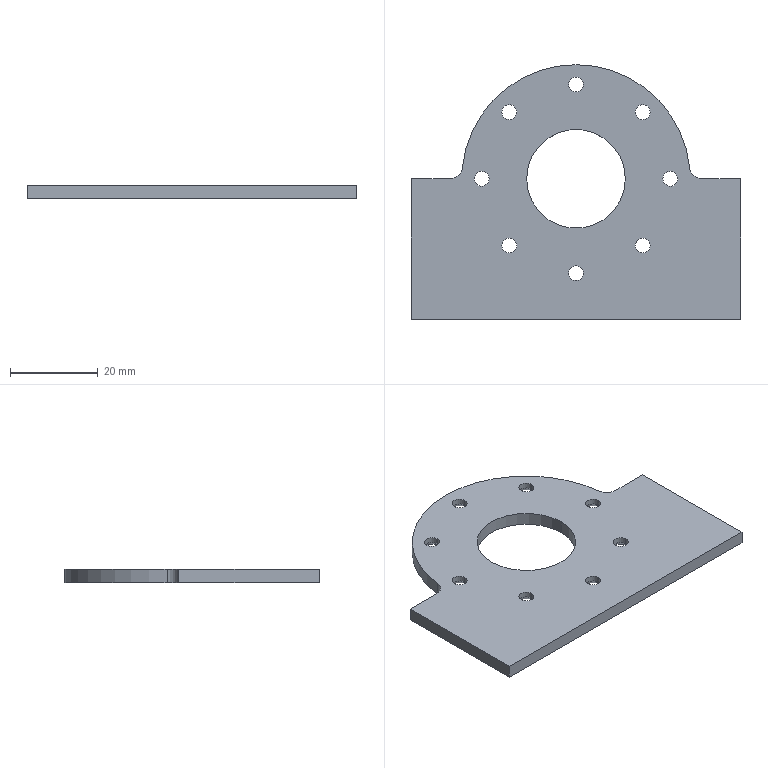Part | SolidWorks | features ICE 2, Extrusion 1, Fillet 1, HoleWzd 1 | 1 solid | 44 faces | box 75 x 58 x 3 mm | volume 8829 mm3 | cylinder 21 | cone 16 | plane 7 | commonest cylinder face diameters 3.4 x16 6 x2 22.5 x2 52 x1
STEP:
#1=CARTESIAN_POINT('',(1.7,37.5,1.66));
#2=VERTEX_POINT('',#1);
#3=CARTESIAN_POINT('',(-1.7,37.5,1.66));
#4=VERTEX_POINT('',#3);
#5=CARTESIAN_POINT('',(0.,37.5,1.66));
#6=DIRECTION('',(0.,0.,-1.));
#7=DIRECTION('',(-1.,0.,0.));
#8=AXIS2_PLACEMENT_3D('',#5,#6,#7);
#9=CIRCLE('',#8,1.7);
#10=EDGE_CURVE('',#2,#4,#9,.T.);
#11=ORIENTED_EDGE('',*,*,#10,.F.);
#12=CARTESIAN_POINT('',(3.36,37.5,0.));
#13=VERTEX_POINT('',#12);
#14=CARTESIAN_POINT('',(3.36,37.5,0.));
#15=DIRECTION('',(0.7071,0.,-0.7071));
#16=VECTOR('',#15,1000.);
#17=LINE('',#14,#16);
#18=EDGE_CURVE('',#2,#13,#17,.T.);
#19=ORIENTED_EDGE('',*,*,#18,.T.);
#20=CARTESIAN_POINT('',(-3.36,37.5,0.));
#21=VERTEX_POINT('',#20);
#22=CARTESIAN_POINT('',(0.,37.5,0.));
#23=DIRECTION('',(0.,0.,-1.));
#24=DIRECTION('',(-1.,0.,0.));
#25=AXIS2_PLACEMENT_3D('',#22,#23,#24);
#26=CIRCLE('',#25,3.36);
#27=EDGE_CURVE('',#13,#21,#26,.T.);
#28=ORIENTED_EDGE('',*,*,#27,.T.);
#29=CARTESIAN_POINT('',(-3.36,37.5,0.));
#30=DIRECTION('',(-0.7071,0.,-0.7071));
#31=VECTOR('',#30,1000.);
#32=LINE('',#29,#31);
#33=EDGE_CURVE('',#4,#21,#32,.T.);
#34=ORIENTED_EDGE('',*,*,#33,.F.);
#35=EDGE_LOOP('',(#11,#19,#28,#34));
#36=FACE_OUTER_BOUND('',#35,.T.);
#37=CARTESIAN_POINT('',(0.,37.5,0.));
#38=DIRECTION('',(0.,0.,-1.));
#39=DIRECTION('',(-1.,0.,0.));
#40=AXIS2_PLACEMENT_3D('',#37,#38,#39);
#41=CONICAL_SURFACE('',#40,3.36,0.7854);
#42=ADVANCED_FACE('',(#36),#41,.F.);
#43=CARTESIAN_POINT('',(1.7,37.5,3.));
#44=VERTEX_POINT('',#43);
#45=CARTESIAN_POINT('',(-1.7,37.5,3.));
#46=VERTEX_POINT('',#45);
#47=CARTESIAN_POINT('',(0.,37.5,3.));
#48=DIRECTION('',(0.,0.,-1.));
#49=DIRECTION('',(-1.,0.,0.));
#50=AXIS2_PLACEMENT_3D('',#47,#48,#49);
#51=CIRCLE('',#50,1.7);
#52=EDGE_CURVE('',#44,#46,#51,.T.);
#53=ORIENTED_EDGE('',*,*,#52,.F.);
#54=CARTESIAN_POINT('',(1.7,37.5,0.));
#55=DIRECTION('',(0.,0.,-1.));
#56=VECTOR('',#55,1000.);
#57=LINE('',#54,#56);
#58=EDGE_CURVE('',#44,#2,#57,.T.);
#59=ORIENTED_EDGE('',*,*,#58,.T.);
#60=ORIENTED_EDGE('',*,*,#10,.T.);
#61=CARTESIAN_POINT('',(-1.7,37.5,0.));
#62=DIRECTION('',(0.,0.,-1.));
#63=VECTOR('',#62,1000.);
#64=LINE('',#61,#63);
#65=EDGE_CURVE('',#46,#4,#64,.T.);
#66=ORIENTED_EDGE('',*,*,#65,.F.);
#67=EDGE_LOOP('',(#53,#59,#60,#66));
#68=FACE_OUTER_BOUND('',#67,.T.);
#69=CARTESIAN_POINT('',(0.,37.5,0.));
#70=DIRECTION('',(0.,0.,-1.));
#71=DIRECTION('',(-1.,0.,0.));
#72=AXIS2_PLACEMENT_3D('',#69,#70,#71);
#73=CYLINDRICAL_SURFACE('',#72,1.7);
#74=ADVANCED_FACE('',(#68),#73,.F.);
#75=CARTESIAN_POINT('',(-13.503,31.203,1.66));
#76=VERTEX_POINT('',#75);
#77=CARTESIAN_POINT('',(-16.903,31.203,1.66));
#78=VERTEX_POINT('',#77);
#79=CARTESIAN_POINT('',(-15.203,31.203,1.66));
#80=DIRECTION('',(0.,0.,-1.));
#81=DIRECTION('',(-1.,0.,0.));
#82=AXIS2_PLACEMENT_3D('',#79,#80,#81);
#83=CIRCLE('',#82,1.7);
#84=EDGE_CURVE('',#76,#78,#83,.T.);
#85=ORIENTED_EDGE('',*,*,#84,.F.);
#86=CARTESIAN_POINT('',(-11.843,31.203,0.));
#87=VERTEX_POINT('',#86);
#88=CARTESIAN_POINT('',(-11.843,31.203,0.));
#89=DIRECTION('',(0.7071,0.,-0.7071));
#90=VECTOR('',#89,1000.);
#91=LINE('',#88,#90);
#92=EDGE_CURVE('',#76,#87,#91,.T.);
#93=ORIENTED_EDGE('',*,*,#92,.T.);
#94=CARTESIAN_POINT('',(-18.563,31.203,0.));
#95=VERTEX_POINT('',#94);
#96=CARTESIAN_POINT('',(-15.203,31.203,0.));
#97=DIRECTION('',(0.,0.,-1.));
#98=DIRECTION('',(-1.,0.,0.));
#99=AXIS2_PLACEMENT_3D('',#96,#97,#98);
#100=CIRCLE('',#99,3.36);
#101=EDGE_CURVE('',#87,#95,#100,.T.);
#102=ORIENTED_EDGE('',*,*,#101,.T.);
#103=CARTESIAN_POINT('',(-18.563,31.203,0.));
#104=DIRECTION('',(-0.7071,0.,-0.7071));
#105=VECTOR('',#104,1000.);
#106=LINE('',#103,#105);
#107=EDGE_CURVE('',#78,#95,#106,.T.);
#108=ORIENTED_EDGE('',*,*,#107,.F.);
#109=EDGE_LOOP('',(#85,#93,#102,#108));
#110=FACE_OUTER_BOUND('',#109,.T.);
#111=CARTESIAN_POINT('',(-15.203,31.203,0.));
#112=DIRECTION('',(0.,0.,-1.));
#113=DIRECTION('',(-1.,0.,0.));
#114=AXIS2_PLACEMENT_3D('',#111,#112,#113);
#115=CONICAL_SURFACE('',#114,3.36,0.7854);
#116=ADVANCED_FACE('',(#110),#115,.F.);
#117=CARTESIAN_POINT('',(-13.503,31.203,3.));
#118=VERTEX_POINT('',#117);
#119=CARTESIAN_POINT('',(-16.903,31.203,3.));
#120=VERTEX_POINT('',#119);
#121=CARTESIAN_POINT('',(-15.203,31.203,3.));
#122=DIRECTION('',(0.,0.,-1.));
#123=DIRECTION('',(-1.,0.,0.));
#124=AXIS2_PLACEMENT_3D('',#121,#122,#123);
#125=CIRCLE('',#124,1.7);
#126=EDGE_CURVE('',#118,#120,#125,.T.);
#127=ORIENTED_EDGE('',*,*,#126,.F.);
#128=CARTESIAN_POINT('',(-13.503,31.203,0.));
#129=DIRECTION('',(0.,0.,-1.));
#130=VECTOR('',#129,1000.);
#131=LINE('',#128,#130);
#132=EDGE_CURVE('',#118,#76,#131,.T.);
#133=ORIENTED_EDGE('',*,*,#132,.T.);
#134=ORIENTED_EDGE('',*,*,#84,.T.);
#135=CARTESIAN_POINT('',(-16.903,31.203,0.));
#136=DIRECTION('',(0.,0.,-1.));
#137=VECTOR('',#136,1000.);
#138=LINE('',#135,#137);
#139=EDGE_CURVE('',#120,#78,#138,.T.);
#140=ORIENTED_EDGE('',*,*,#139,.F.);
#141=EDGE_LOOP('',(#127,#133,#134,#140));
#142=FACE_OUTER_BOUND('',#141,.T.);
#143=CARTESIAN_POINT('',(-15.203,31.203,0.));
#144=DIRECTION('',(0.,0.,-1.));
#145=DIRECTION('',(-1.,0.,0.));
#146=AXIS2_PLACEMENT_3D('',#143,#144,#145);
#147=CYLINDRICAL_SURFACE('',#146,1.7);
#148=ADVANCED_FACE('',(#142),#147,.F.);
#149=CARTESIAN_POINT('',(-19.8,16.,1.66));
#150=VERTEX_POINT('',#149);
#151=CARTESIAN_POINT('',(-23.2,16.,1.66));
#152=VERTEX_POINT('',#151);
#153=CARTESIAN_POINT('',(-21.5,16.,1.66));
#154=DIRECTION('',(0.,0.,-1.));
#155=DIRECTION('',(-1.,0.,0.));
#156=AXIS2_PLACEMENT_3D('',#153,#154,#155);
#157=CIRCLE('',#156,1.7);
#158=EDGE_CURVE('',#150,#152,#157,.T.);
#159=ORIENTED_EDGE('',*,*,#158,.F.);
#160=CARTESIAN_POINT('',(-18.14,16.,0.));
#161=VERTEX_POINT('',#160);
#162=CARTESIAN_POINT('',(-18.14,16.,0.));
#163=DIRECTION('',(0.7071,0.,-0.7071));
#164=VECTOR('',#163,1000.);
#165=LINE('',#162,#164);
#166=EDGE_CURVE('',#150,#161,#165,.T.);
#167=ORIENTED_EDGE('',*,*,#166,.T.);
#168=CARTESIAN_POINT('',(-24.86,16.,0.));
#169=VERTEX_POINT('',#168);
#170=CARTESIAN_POINT('',(-21.5,16.,0.));
#171=DIRECTION('',(0.,0.,-1.));
#172=DIRECTION('',(-1.,0.,0.));
#173=AXIS2_PLACEMENT_3D('',#170,#171,#172);
#174=CIRCLE('',#173,3.36);
#175=EDGE_CURVE('',#161,#169,#174,.T.);
#176=ORIENTED_EDGE('',*,*,#175,.T.);
#177=CARTESIAN_POINT('',(-24.86,16.,0.));
#178=DIRECTION('',(-0.7071,0.,-0.7071));
#179=VECTOR('',#178,1000.);
#180=LINE('',#177,#179);
#181=EDGE_CURVE('',#152,#169,#180,.T.);
#182=ORIENTED_EDGE('',*,*,#181,.F.);
#183=EDGE_LOOP('',(#159,#167,#176,#182));
#184=FACE_OUTER_BOUND('',#183,.T.);
#185=CARTESIAN_POINT('',(-21.5,16.,0.));
#186=DIRECTION('',(0.,0.,-1.));
#187=DIRECTION('',(-1.,0.,0.));
#188=AXIS2_PLACEMENT_3D('',#185,#186,#187);
#189=CONICAL_SURFACE('',#188,3.36,0.7854);
#190=ADVANCED_FACE('',(#184),#189,.F.);
#191=CARTESIAN_POINT('',(-19.8,16.,3.));
#192=VERTEX_POINT('',#191);
#193=CARTESIAN_POINT('',(-23.2,16.,3.));
#194=VERTEX_POINT('',#193);
#195=CARTESIAN_POINT('',(-21.5,16.,3.));
#196=DIRECTION('',(0.,0.,-1.));
#197=DIRECTION('',(-1.,0.,0.));
#198=AXIS2_PLACEMENT_3D('',#195,#196,#197);
#199=CIRCLE('',#198,1.7);
#200=EDGE_CURVE('',#192,#194,#199,.T.);
#201=ORIENTED_EDGE('',*,*,#200,.F.);
#202=CARTESIAN_POINT('',(-19.8,16.,0.));
#203=DIRECTION('',(0.,0.,-1.));
#204=VECTOR('',#203,1000.);
#205=LINE('',#202,#204);
#206=EDGE_CURVE('',#192,#150,#205,.T.);
#207=ORIENTED_EDGE('',*,*,#206,.T.);
#208=ORIENTED_EDGE('',*,*,#158,.T.);
#209=CARTESIAN_POINT('',(-23.2,16.,0.));
#210=DIRECTION('',(0.,0.,-1.));
#211=VECTOR('',#210,1000.);
#212=LINE('',#209,#211);
#213=EDGE_CURVE('',#194,#152,#212,.T.);
#214=ORIENTED_EDGE('',*,*,#213,.F.);
#215=EDGE_LOOP('',(#201,#207,#208,#214));
#216=FACE_OUTER_BOUND('',#215,.T.);
#217=CARTESIAN_POINT('',(-21.5,16.,0.));
#218=DIRECTION('',(0.,0.,-1.));
#219=DIRECTION('',(-1.,0.,0.));
#220=AXIS2_PLACEMENT_3D('',#217,#218,#219);
#221=CYLINDRICAL_SURFACE('',#220,1.7);
#222=ADVANCED_FACE('',(#216),#221,.F.);
#223=CARTESIAN_POINT('',(-13.503,0.7972,1.66));
#224=VERTEX_POINT('',#223);
#225=CARTESIAN_POINT('',(-16.903,0.7972,1.66));
#226=VERTEX_POINT('',#225);
#227=CARTESIAN_POINT('',(-15.203,0.7972,1.66));
#228=DIRECTION('',(0.,0.,-1.));
#229=DIRECTION('',(-1.,0.,0.));
#230=AXIS2_PLACEMENT_3D('',#227,#228,#229);
#231=CIRCLE('',#230,1.7);
#232=EDGE_CURVE('',#224,#226,#231,.T.);
#233=ORIENTED_EDGE('',*,*,#232,.F.);
#234=CARTESIAN_POINT('',(-11.843,0.7972,0.));
#235=VERTEX_POINT('',#234);
#236=CARTESIAN_POINT('',(-11.843,0.7972,0.));
#237=DIRECTION('',(0.7071,0.,-0.7071));
#238=VECTOR('',#237,1000.);
#239=LINE('',#236,#238);
#240=EDGE_CURVE('',#224,#235,#239,.T.);
#241=ORIENTED_EDGE('',*,*,#240,.T.);
#242=CARTESIAN_POINT('',(-18.563,0.7972,0.));
#243=VERTEX_POINT('',#242);
#244=CARTESIAN_POINT('',(-15.203,0.7972,0.));
#245=DIRECTION('',(0.,0.,-1.));
#246=DIRECTION('',(-1.,0.,0.));
#247=AXIS2_PLACEMENT_3D('',#244,#245,#246);
#248=CIRCLE('',#247,3.36);
#249=EDGE_CURVE('',#235,#243,#248,.T.);
#250=ORIENTED_EDGE('',*,*,#249,.T.);
#251=CARTESIAN_POINT('',(-18.563,0.7972,0.));
#252=DIRECTION('',(-0.7071,0.,-0.7071));
#253=VECTOR('',#252,1000.);
#254=LINE('',#251,#253);
#255=EDGE_CURVE('',#226,#243,#254,.T.);
#256=ORIENTED_EDGE('',*,*,#255,.F.);
#257=EDGE_LOOP('',(#233,#241,#250,#256));
#258=FACE_OUTER_BOUND('',#257,.T.);
#259=CARTESIAN_POINT('',(-15.203,0.7972,0.));
#260=DIRECTION('',(0.,0.,-1.));
#261=DIRECTION('',(-1.,0.,0.));
#262=AXIS2_PLACEMENT_3D('',#259,#260,#261);
#263=CONICAL_SURFACE('',#262,3.36,0.7854);
#264=ADVANCED_FACE('',(#258),#263,.F.);
#265=CARTESIAN_POINT('',(-13.503,0.7972,3.));
#266=VERTEX_POINT('',#265);
#267=CARTESIAN_POINT('',(-16.903,0.7972,3.));
#268=VERTEX_POINT('',#267);
#269=CARTESIAN_POINT('',(-15.203,0.7972,3.));
#270=DIRECTION('',(0.,0.,-1.));
#271=DIRECTION('',(-1.,0.,0.));
#272=AXIS2_PLACEMENT_3D('',#269,#270,#271);
#273=CIRCLE('',#272,1.7);
#274=EDGE_CURVE('',#266,#268,#273,.T.);
#275=ORIENTED_EDGE('',*,*,#274,.F.);
#276=CARTESIAN_POINT('',(-13.503,0.7972,0.));
#277=DIRECTION('',(0.,0.,-1.));
#278=VECTOR('',#277,1000.);
#279=LINE('',#276,#278);
#280=EDGE_CURVE('',#266,#224,#279,.T.);
#281=ORIENTED_EDGE('',*,*,#280,.T.);
#282=ORIENTED_EDGE('',*,*,#232,.T.);
#283=CARTESIAN_POINT('',(-16.903,0.7972,0.));
#284=DIRECTION('',(0.,0.,-1.));
#285=VECTOR('',#284,1000.);
#286=LINE('',#283,#285);
#287=EDGE_CURVE('',#268,#226,#286,.T.);
#288=ORIENTED_EDGE('',*,*,#287,.F.);
#289=EDGE_LOOP('',(#275,#281,#282,#288));
#290=FACE_OUTER_BOUND('',#289,.T.);
#291=CARTESIAN_POINT('',(-15.203,0.7972,0.));
#292=DIRECTION('',(0.,0.,-1.));
#293=DIRECTION('',(-1.,0.,0.));
#294=AXIS2_PLACEMENT_3D('',#291,#292,#293);
#295=CYLINDRICAL_SURFACE('',#294,1.7);
#296=ADVANCED_FACE('',(#290),#295,.F.);
#297=CARTESIAN_POINT('',(1.7,-5.5,1.66));
#298=VERTEX_POINT('',#297);
#299=CARTESIAN_POINT('',(-1.7,-5.5,1.66));
#300=VERTEX_POINT('',#299);
#301=CARTESIAN_POINT('',(0.,-5.5,1.66));
#302=DIRECTION('',(0.,0.,-1.));
#303=DIRECTION('',(-1.,0.,0.));
#304=AXIS2_PLACEMENT_3D('',#301,#302,#303);
#305=CIRCLE('',#304,1.7);
#306=EDGE_CURVE('',#298,#300,#305,.T.);
#307=ORIENTED_EDGE('',*,*,#306,.F.);
#308=CARTESIAN_POINT('',(3.36,-5.5,0.));
#309=VERTEX_POINT('',#308);
#310=CARTESIAN_POINT('',(3.36,-5.5,0.));
#311=DIRECTION('',(0.7071,0.,-0.7071));
#312=VECTOR('',#311,1000.);
#313=LINE('',#310,#312);
#314=EDGE_CURVE('',#298,#309,#313,.T.);
#315=ORIENTED_EDGE('',*,*,#314,.T.);
#316=CARTESIAN_POINT('',(-3.36,-5.5,0.));
#317=VERTEX_POINT('',#316);
#318=CARTESIAN_POINT('',(0.,-5.5,0.));
#319=DIRECTION('',(0.,0.,-1.));
#320=DIRECTION('',(-1.,0.,0.));
#321=AXIS2_PLACEMENT_3D('',#318,#319,#320);
#322=CIRCLE('',#321,3.36);
#323=EDGE_CURVE('',#309,#317,#322,.T.);
#324=ORIENTED_EDGE('',*,*,#323,.T.);
#325=CARTESIAN_POINT('',(-3.36,-5.5,0.));
#326=DIRECTION('',(-0.7071,0.,-0.7071));
#327=VECTOR('',#326,1000.);
#328=LINE('',#325,#327);
#329=EDGE_CURVE('',#300,#317,#328,.T.);
#330=ORIENTED_EDGE('',*,*,#329,.F.);
#331=EDGE_LOOP('',(#307,#315,#324,#330));
#332=FACE_OUTER_BOUND('',#331,.T.);
#333=CARTESIAN_POINT('',(0.,-5.5,0.));
#334=DIRECTION('',(0.,0.,-1.));
#335=DIRECTION('',(-1.,0.,0.));
#336=AXIS2_PLACEMENT_3D('',#333,#334,#335);
#337=CONICAL_SURFACE('',#336,3.36,0.7854);
#338=ADVANCED_FACE('',(#332),#337,.F.);
#339=CARTESIAN_POINT('',(1.7,-5.5,3.));
#340=VERTEX_POINT('',#339);
#341=CARTESIAN_POINT('',(-1.7,-5.5,3.));
#342=VERTEX_POINT('',#341);
#343=CARTESIAN_POINT('',(0.,-5.5,3.));
#344=DIRECTION('',(0.,0.,-1.));
#345=DIRECTION('',(-1.,0.,0.));
#346=AXIS2_PLACEMENT_3D('',#343,#344,#345);
#347=CIRCLE('',#346,1.7);
#348=EDGE_CURVE('',#340,#342,#347,.T.);
#349=ORIENTED_EDGE('',*,*,#348,.F.);
#350=CARTESIAN_POINT('',(1.7,-5.5,0.));
#351=DIRECTION('',(0.,0.,-1.));
#352=VECTOR('',#351,1000.);
#353=LINE('',#350,#352);
#354=EDGE_CURVE('',#340,#298,#353,.T.);
#355=ORIENTED_EDGE('',*,*,#354,.T.);
#356=ORIENTED_EDGE('',*,*,#306,.T.);
#357=CARTESIAN_POINT('',(-1.7,-5.5,0.));
#358=DIRECTION('',(0.,0.,-1.));
#359=VECTOR('',#358,1000.);
#360=LINE('',#357,#359);
#361=EDGE_CURVE('',#342,#300,#360,.T.);
#362=ORIENTED_EDGE('',*,*,#361,.F.);
#363=EDGE_LOOP('',(#349,#355,#356,#362));
#364=FACE_OUTER_BOUND('',#363,.T.);
#365=CARTESIAN_POINT('',(0.,-5.5,0.));
#366=DIRECTION('',(0.,0.,-1.));
#367=DIRECTION('',(-1.,0.,0.));
#368=AXIS2_PLACEMENT_3D('',#365,#366,#367);
#369=CYLINDRICAL_SURFACE('',#368,1.7);
#370=ADVANCED_FACE('',(#364),#369,.F.);
#371=CARTESIAN_POINT('',(16.903,0.7972,1.66));
#372=VERTEX_POINT('',#371);
#373=CARTESIAN_POINT('',(13.503,0.7972,1.66));
#374=VERTEX_POINT('',#373);
#375=CARTESIAN_POINT('',(15.203,0.7972,1.66));
#376=DIRECTION('',(0.,0.,-1.));
#377=DIRECTION('',(-1.,0.,0.));
#378=AXIS2_PLACEMENT_3D('',#375,#376,#377);
#379=CIRCLE('',#378,1.7);
#380=EDGE_CURVE('',#372,#374,#379,.T.);
#381=ORIENTED_EDGE('',*,*,#380,.F.);
#382=CARTESIAN_POINT('',(18.563,0.7972,0.));
#383=VERTEX_POINT('',#382);
#384=CARTESIAN_POINT('',(18.563,0.7972,0.));
#385=DIRECTION('',(0.7071,0.,-0.7071));
#386=VECTOR('',#385,1000.);
#387=LINE('',#384,#386);
#388=EDGE_CURVE('',#372,#383,#387,.T.);
#389=ORIENTED_EDGE('',*,*,#388,.T.);
#390=CARTESIAN_POINT('',(11.843,0.7972,0.));
#391=VERTEX_POINT('',#390);
#392=CARTESIAN_POINT('',(15.203,0.7972,0.));
#393=DIRECTION('',(0.,0.,-1.));
#394=DIRECTION('',(-1.,0.,0.));
#395=AXIS2_PLACEMENT_3D('',#392,#393,#394);
#396=CIRCLE('',#395,3.36);
#397=EDGE_CURVE('',#383,#391,#396,.T.);
#398=ORIENTED_EDGE('',*,*,#397,.T.);
#399=CARTESIAN_POINT('',(11.843,0.7972,0.));
#400=DIRECTION('',(-0.7071,0.,-0.7071));
#401=VECTOR('',#400,1000.);
#402=LINE('',#399,#401);
#403=EDGE_CURVE('',#374,#391,#402,.T.);
#404=ORIENTED_EDGE('',*,*,#403,.F.);
#405=EDGE_LOOP('',(#381,#389,#398,#404));
#406=FACE_OUTER_BOUND('',#405,.T.);
#407=CARTESIAN_POINT('',(15.203,0.7972,0.));
#408=DIRECTION('',(0.,0.,-1.));
#409=DIRECTION('',(-1.,0.,0.));
#410=AXIS2_PLACEMENT_3D('',#407,#408,#409);
#411=CONICAL_SURFACE('',#410,3.36,0.7854);
#412=ADVANCED_FACE('',(#406),#411,.F.);
#413=CARTESIAN_POINT('',(16.903,0.7972,3.));
#414=VERTEX_POINT('',#413);
#415=CARTESIAN_POINT('',(13.503,0.7972,3.));
#416=VERTEX_POINT('',#415);
#417=CARTESIAN_POINT('',(15.203,0.7972,3.));
#418=DIRECTION('',(0.,0.,-1.));
#419=DIRECTION('',(-1.,0.,0.));
#420=AXIS2_PLACEMENT_3D('',#417,#418,#419);
#421=CIRCLE('',#420,1.7);
#422=EDGE_CURVE('',#414,#416,#421,.T.);
#423=ORIENTED_EDGE('',*,*,#422,.F.);
#424=CARTESIAN_POINT('',(16.903,0.7972,0.));
#425=DIRECTION('',(0.,0.,-1.));
#426=VECTOR('',#425,1000.);
#427=LINE('',#424,#426);
#428=EDGE_CURVE('',#414,#372,#427,.T.);
#429=ORIENTED_EDGE('',*,*,#428,.T.);
#430=ORIENTED_EDGE('',*,*,#380,.T.);
#431=CARTESIAN_POINT('',(13.503,0.7972,0.));
#432=DIRECTION('',(0.,0.,-1.));
#433=VECTOR('',#432,1000.);
#434=LINE('',#431,#433);
#435=EDGE_CURVE('',#416,#374,#434,.T.);
#436=ORIENTED_EDGE('',*,*,#435,.F.);
#437=EDGE_LOOP('',(#423,#429,#430,#436));
#438=FACE_OUTER_BOUND('',#437,.T.);
#439=CARTESIAN_POINT('',(15.203,0.7972,0.));
#440=DIRECTION('',(0.,0.,-1.));
#441=DIRECTION('',(-1.,0.,0.));
#442=AXIS2_PLACEMENT_3D('',#439,#440,#441);
#443=CYLINDRICAL_SURFACE('',#442,1.7);
#444=ADVANCED_FACE('',(#438),#443,.F.);
#445=CARTESIAN_POINT('',(23.2,16.,1.66));
#446=VERTEX_POINT('',#445);
#447=CARTESIAN_POINT('',(19.8,16.,1.66));
#448=VERTEX_POINT('',#447);
#449=CARTESIAN_POINT('',(21.5,16.,1.66));
#450=DIRECTION('',(0.,0.,-1.));
#451=DIRECTION('',(-1.,0.,0.));
#452=AXIS2_PLACEMENT_3D('',#449,#450,#451);
#453=CIRCLE('',#452,1.7);
#454=EDGE_CURVE('',#446,#448,#453,.T.);
#455=ORIENTED_EDGE('',*,*,#454,.F.);
#456=CARTESIAN_POINT('',(24.86,16.,0.));
#457=VERTEX_POINT('',#456);
#458=CARTESIAN_POINT('',(24.86,16.,0.));
#459=DIRECTION('',(0.7071,0.,-0.7071));
#460=VECTOR('',#459,1000.);
#461=LINE('',#458,#460);
#462=EDGE_CURVE('',#446,#457,#461,.T.);
#463=ORIENTED_EDGE('',*,*,#462,.T.);
#464=CARTESIAN_POINT('',(18.14,16.,0.));
#465=VERTEX_POINT('',#464);
#466=CARTESIAN_POINT('',(21.5,16.,0.));
#467=DIRECTION('',(0.,0.,-1.));
#468=DIRECTION('',(-1.,0.,0.));
#469=AXIS2_PLACEMENT_3D('',#466,#467,#468);
#470=CIRCLE('',#469,3.36);
#471=EDGE_CURVE('',#457,#465,#470,.T.);
#472=ORIENTED_EDGE('',*,*,#471,.T.);
#473=CARTESIAN_POINT('',(18.14,16.,0.));
#474=DIRECTION('',(-0.7071,0.,-0.7071));
#475=VECTOR('',#474,1000.);
#476=LINE('',#473,#475);
#477=EDGE_CURVE('',#448,#465,#476,.T.);
#478=ORIENTED_EDGE('',*,*,#477,.F.);
#479=EDGE_LOOP('',(#455,#463,#472,#478));
#480=FACE_OUTER_BOUND('',#479,.T.);
#481=CARTESIAN_POINT('',(21.5,16.,0.));
#482=DIRECTION('',(0.,0.,-1.));
#483=DIRECTION('',(-1.,0.,0.));
#484=AXIS2_PLACEMENT_3D('',#481,#482,#483);
#485=CONICAL_SURFACE('',#484,3.36,0.7854);
#486=ADVANCED_FACE('',(#480),#485,.F.);
#487=CARTESIAN_POINT('',(23.2,16.,3.));
#488=VERTEX_POINT('',#487);
#489=CARTESIAN_POINT('',(19.8,16.,3.));
#490=VERTEX_POINT('',#489);
#491=CARTESIAN_POINT('',(21.5,16.,3.));
#492=DIRECTION('',(0.,0.,-1.));
#493=DIRECTION('',(-1.,0.,0.));
#494=AXIS2_PLACEMENT_3D('',#491,#492,#493);
#495=CIRCLE('',#494,1.7);
#496=EDGE_CURVE('',#488,#490,#495,.T.);
#497=ORIENTED_EDGE('',*,*,#496,.F.);
#498=CARTESIAN_POINT('',(23.2,16.,0.));
#499=DIRECTION('',(0.,0.,-1.));
#500=VECTOR('',#499,1000.);
#501=LINE('',#498,#500);
#502=EDGE_CURVE('',#488,#446,#501,.T.);
#503=ORIENTED_EDGE('',*,*,#502,.T.);
#504=ORIENTED_EDGE('',*,*,#454,.T.);
#505=CARTESIAN_POINT('',(19.8,16.,0.));
#506=DIRECTION('',(0.,0.,-1.));
#507=VECTOR('',#506,1000.);
#508=LINE('',#505,#507);
#509=EDGE_CURVE('',#490,#448,#508,.T.);
#510=ORIENTED_EDGE('',*,*,#509,.F.);
#511=EDGE_LOOP('',(#497,#503,#504,#510));
#512=FACE_OUTER_BOUND('',#511,.T.);
#513=CARTESIAN_POINT('',(21.5,16.,0.));
#514=DIRECTION('',(0.,0.,-1.));
#515=DIRECTION('',(-1.,0.,0.));
#516=AXIS2_PLACEMENT_3D('',#513,#514,#515);
#517=CYLINDRICAL_SURFACE('',#516,1.7);
#518=ADVANCED_FACE('',(#512),#517,.F.);
#519=CARTESIAN_POINT('',(16.903,31.203,1.66));
#520=VERTEX_POINT('',#519);
#521=CARTESIAN_POINT('',(13.503,31.203,1.66));
#522=VERTEX_POINT('',#521);
#523=CARTESIAN_POINT('',(15.203,31.203,1.66));
#524=DIRECTION('',(0.,0.,-1.));
#525=DIRECTION('',(-1.,0.,0.));
#526=AXIS2_PLACEMENT_3D('',#523,#524,#525);
#527=CIRCLE('',#526,1.7);
#528=EDGE_CURVE('',#520,#522,#527,.T.);
#529=ORIENTED_EDGE('',*,*,#528,.F.);
#530=CARTESIAN_POINT('',(18.563,31.203,0.));
#531=VERTEX_POINT('',#530);
#532=CARTESIAN_POINT('',(18.563,31.203,0.));
#533=DIRECTION('',(0.7071,0.,-0.7071));
#534=VECTOR('',#533,1000.);
#535=LINE('',#532,#534);
#536=EDGE_CURVE('',#520,#531,#535,.T.);
#537=ORIENTED_EDGE('',*,*,#536,.T.);
#538=CARTESIAN_POINT('',(11.843,31.203,0.));
#539=VERTEX_POINT('',#538);
#540=CARTESIAN_POINT('',(15.203,31.203,0.));
#541=DIRECTION('',(0.,0.,-1.));
#542=DIRECTION('',(-1.,0.,0.));
#543=AXIS2_PLACEMENT_3D('',#540,#541,#542);
#544=CIRCLE('',#543,3.36);
#545=EDGE_CURVE('',#531,#539,#544,.T.);
#546=ORIENTED_EDGE('',*,*,#545,.T.);
#547=CARTESIAN_POINT('',(11.843,31.203,0.));
#548=DIRECTION('',(-0.7071,0.,-0.7071));
#549=VECTOR('',#548,1000.);
#550=LINE('',#547,#549);
#551=EDGE_CURVE('',#522,#539,#550,.T.);
#552=ORIENTED_EDGE('',*,*,#551,.F.);
#553=EDGE_LOOP('',(#529,#537,#546,#552));
#554=FACE_OUTER_BOUND('',#553,.T.);
#555=CARTESIAN_POINT('',(15.203,31.203,0.));
#556=DIRECTION('',(0.,0.,-1.));
#557=DIRECTION('',(-1.,0.,0.));
#558=AXIS2_PLACEMENT_3D('',#555,#556,#557);
#559=CONICAL_SURFACE('',#558,3.36,0.7854);
#560=ADVANCED_FACE('',(#554),#559,.F.);
#561=CARTESIAN_POINT('',(16.903,31.203,3.));
#562=VERTEX_POINT('',#561);
#563=CARTESIAN_POINT('',(13.503,31.203,3.));
#564=VERTEX_POINT('',#563);
#565=CARTESIAN_POINT('',(15.203,31.203,3.));
#566=DIRECTION('',(0.,0.,-1.));
#567=DIRECTION('',(-1.,0.,0.));
#568=AXIS2_PLACEMENT_3D('',#565,#566,#567);
#569=CIRCLE('',#568,1.7);
#570=EDGE_CURVE('',#562,#564,#569,.T.);
#571=ORIENTED_EDGE('',*,*,#570,.F.);
#572=CARTESIAN_POINT('',(16.903,31.203,0.));
#573=DIRECTION('',(0.,0.,-1.));
#574=VECTOR('',#573,1000.);
#575=LINE('',#572,#574);
#576=EDGE_CURVE('',#562,#520,#575,.T.);
#577=ORIENTED_EDGE('',*,*,#576,.T.);
#578=ORIENTED_EDGE('',*,*,#528,.T.);
#579=CARTESIAN_POINT('',(13.503,31.203,0.));
#580=DIRECTION('',(0.,0.,-1.));
#581=VECTOR('',#580,1000.);
#582=LINE('',#579,#581);
#583=EDGE_CURVE('',#564,#522,#582,.T.);
#584=ORIENTED_EDGE('',*,*,#583,.F.);
#585=EDGE_LOOP('',(#571,#577,#578,#584));
#586=FACE_OUTER_BOUND('',#585,.T.);
#587=CARTESIAN_POINT('',(15.203,31.203,0.));
#588=DIRECTION('',(0.,0.,-1.));
#589=DIRECTION('',(-1.,0.,0.));
#590=AXIS2_PLACEMENT_3D('',#587,#588,#589);
#591=CYLINDRICAL_SURFACE('',#590,1.7);
#592=ADVANCED_FACE('',(#586),#591,.F.);
#593=CARTESIAN_POINT('',(11.25,16.,3.));
#594=VERTEX_POINT('',#593);
#595=CARTESIAN_POINT('',(-11.25,16.,3.));
#596=VERTEX_POINT('',#595);
#597=CARTESIAN_POINT('',(0.,16.,3.));
#598=DIRECTION('',(0.,0.,-1.));
#599=DIRECTION('',(-1.,0.,0.));
#600=AXIS2_PLACEMENT_3D('',#597,#598,#599);
#601=CIRCLE('',#600,11.25);
#602=EDGE_CURVE('',#594,#596,#601,.T.);
#603=ORIENTED_EDGE('',*,*,#602,.F.);
#604=CARTESIAN_POINT('',(11.25,16.,0.));
#605=VERTEX_POINT('',#604);
#606=CARTESIAN_POINT('',(11.25,16.,3.));
#607=DIRECTION('',(0.,0.,-1.));
#608=VECTOR('',#607,1000.);
#609=LINE('',#606,#608);
#610=EDGE_CURVE('',#594,#605,#609,.T.);
#611=ORIENTED_EDGE('',*,*,#610,.T.);
#612=CARTESIAN_POINT('',(-11.25,16.,0.));
#613=VERTEX_POINT('',#612);
#614=CARTESIAN_POINT('',(0.,16.,0.));
#615=DIRECTION('',(0.,0.,-1.));
#616=DIRECTION('',(-1.,0.,0.));
#617=AXIS2_PLACEMENT_3D('',#614,#615,#616);
#618=CIRCLE('',#617,11.25);
#619=EDGE_CURVE('',#605,#613,#618,.T.);
#620=ORIENTED_EDGE('',*,*,#619,.T.);
#621=CARTESIAN_POINT('',(-11.25,16.,3.));
#622=DIRECTION('',(0.,0.,-1.));
#623=VECTOR('',#622,1000.);
#624=LINE('',#621,#623);
#625=EDGE_CURVE('',#596,#613,#624,.T.);
#626=ORIENTED_EDGE('',*,*,#625,.F.);
#627=EDGE_LOOP('',(#603,#611,#620,#626));
#628=FACE_OUTER_BOUND('',#627,.T.);
#629=CARTESIAN_POINT('',(0.,16.,3.));
#630=DIRECTION('',(0.,0.,-1.));
#631=DIRECTION('',(-1.,0.,0.));
#632=AXIS2_PLACEMENT_3D('',#629,#630,#631);
#633=CYLINDRICAL_SURFACE('',#632,11.25);
#634=ADVANCED_FACE('',(#628),#633,.F.);
#635=CARTESIAN_POINT('',(37.5,16.,0.));
#636=VERTEX_POINT('',#635);
#637=CARTESIAN_POINT('',(28.844,16.,0.));
#638=VERTEX_POINT('',#637);
#639=CARTESIAN_POINT('',(-37.5,16.,0.));
#640=DIRECTION('',(-1.,0.,0.));
#641=VECTOR('',#640,1000.);
#642=LINE('',#639,#641);
#643=EDGE_CURVE('',#636,#638,#642,.T.);
#644=ORIENTED_EDGE('',*,*,#643,.T.);
#645=CARTESIAN_POINT('',(28.844,16.,3.));
#646=VERTEX_POINT('',#645);
#647=CARTESIAN_POINT('',(28.844,16.,3.));
#648=DIRECTION('',(0.,0.,1.));
#649=VECTOR('',#648,1000.);
#650=LINE('',#647,#649);
#651=EDGE_CURVE('',#638,#646,#650,.T.);
#652=ORIENTED_EDGE('',*,*,#651,.T.);
#653=CARTESIAN_POINT('',(37.5,16.,3.));
#654=VERTEX_POINT('',#653);
#655=CARTESIAN_POINT('',(-37.5,16.,3.));
#656=DIRECTION('',(-1.,0.,0.));
#657=VECTOR('',#656,1000.);
#658=LINE('',#655,#657);
#659=EDGE_CURVE('',#654,#646,#658,.T.);
#660=ORIENTED_EDGE('',*,*,#659,.F.);
#661=CARTESIAN_POINT('',(37.5,16.,3.));
#662=DIRECTION('',(0.,0.,-1.));
#663=VECTOR('',#662,1000.);
#664=LINE('',#661,#663);
#665=EDGE_CURVE('',#654,#636,#664,.T.);
#666=ORIENTED_EDGE('',*,*,#665,.T.);
#667=EDGE_LOOP('',(#644,#652,#660,#666));
#668=FACE_OUTER_BOUND('',#667,.T.);
#669=CARTESIAN_POINT('',(-37.5,16.,3.));
#670=DIRECTION('',(0.,-1.,0.));
#671=DIRECTION('',(0.,0.,-1.));
#672=AXIS2_PLACEMENT_3D('',#669,#670,#671);
#673=PLANE('',#672);
#674=ADVANCED_FACE('',(#668),#673,.F.);
#675=CARTESIAN_POINT('',(37.5,-16.,0.));
#676=VERTEX_POINT('',#675);
#677=CARTESIAN_POINT('',(37.5,-16.,0.));
#678=DIRECTION('',(0.,1.,0.));
#679=VECTOR('',#678,1000.);
#680=LINE('',#677,#679);
#681=EDGE_CURVE('',#676,#636,#680,.T.);
#682=ORIENTED_EDGE('',*,*,#681,.T.);
#683=ORIENTED_EDGE('',*,*,#665,.F.);
#684=CARTESIAN_POINT('',(37.5,-16.,3.));
#685=VERTEX_POINT('',#684);
#686=CARTESIAN_POINT('',(37.5,-16.,3.));
#687=DIRECTION('',(0.,1.,0.));
#688=VECTOR('',#687,1000.);
#689=LINE('',#686,#688);
#690=EDGE_CURVE('',#685,#654,#689,.T.);
#691=ORIENTED_EDGE('',*,*,#690,.F.);
#692=CARTESIAN_POINT('',(37.5,-16.,3.));
#693=DIRECTION('',(0.,0.,-1.));
#694=VECTOR('',#693,1000.);
#695=LINE('',#692,#694);
#696=EDGE_CURVE('',#685,#676,#695,.T.);
#697=ORIENTED_EDGE('',*,*,#696,.T.);
#698=EDGE_LOOP('',(#682,#683,#691,#697));
#699=FACE_OUTER_BOUND('',#698,.T.);
#700=CARTESIAN_POINT('',(37.5,-16.,3.));
#701=DIRECTION('',(-1.,0.,0.));
#702=DIRECTION('',(0.,0.,1.));
#703=AXIS2_PLACEMENT_3D('',#700,#701,#702);
#704=PLANE('',#703);
#705=ADVANCED_FACE('',(#699),#704,.F.);
#706=CARTESIAN_POINT('',(-28.844,16.,3.));
#707=VERTEX_POINT('',#706);
#708=CARTESIAN_POINT('',(-37.5,16.,3.));
#709=VERTEX_POINT('',#708);
#710=CARTESIAN_POINT('',(-37.5,16.,3.));
#711=DIRECTION('',(-1.,0.,0.));
#712=VECTOR('',#711,1000.);
#713=LINE('',#710,#712);
#714=EDGE_CURVE('',#707,#709,#713,.T.);
#715=ORIENTED_EDGE('',*,*,#714,.F.);
#716=CARTESIAN_POINT('',(-28.844,16.,0.));
#717=VERTEX_POINT('',#716);
#718=CARTESIAN_POINT('',(-28.844,16.,3.));
#719=DIRECTION('',(0.,0.,-1.));
#720=VECTOR('',#719,1000.);
#721=LINE('',#718,#720);
#722=EDGE_CURVE('',#707,#717,#721,.T.);
#723=ORIENTED_EDGE('',*,*,#722,.T.);
#724=CARTESIAN_POINT('',(-37.5,16.,0.));
#725=VERTEX_POINT('',#724);
#726=CARTESIAN_POINT('',(-37.5,16.,0.));
#727=DIRECTION('',(-1.,0.,0.));
#728=VECTOR('',#727,1000.);
#729=LINE('',#726,#728);
#730=EDGE_CURVE('',#717,#725,#729,.T.);
#731=ORIENTED_EDGE('',*,*,#730,.T.);
#732=CARTESIAN_POINT('',(-37.5,16.,3.));
#733=DIRECTION('',(0.,0.,-1.));
#734=VECTOR('',#733,1000.);
#735=LINE('',#732,#734);
#736=EDGE_CURVE('',#709,#725,#735,.T.);
#737=ORIENTED_EDGE('',*,*,#736,.F.);
#738=EDGE_LOOP('',(#715,#723,#731,#737));
#739=FACE_OUTER_BOUND('',#738,.T.);
#740=CARTESIAN_POINT('',(-37.5,16.,3.));
#741=DIRECTION('',(0.,-1.,0.));
#742=DIRECTION('',(0.,0.,-1.));
#743=AXIS2_PLACEMENT_3D('',#740,#741,#742);
#744=PLANE('',#743);
#745=ADVANCED_FACE('',(#739),#744,.F.);
#746=CARTESIAN_POINT('',(-37.5,-16.,0.));
#747=VERTEX_POINT('',#746);
#748=CARTESIAN_POINT('',(-37.5,-16.,0.));
#749=DIRECTION('',(0.,-1.,0.));
#750=VECTOR('',#749,1000.);
#751=LINE('',#748,#750);
#752=EDGE_CURVE('',#725,#747,#751,.T.);
#753=ORIENTED_EDGE('',*,*,#752,.T.);
#754=CARTESIAN_POINT('',(-37.5,-16.,3.));
#755=VERTEX_POINT('',#754);
#756=CARTESIAN_POINT('',(-37.5,-16.,3.));
#757=DIRECTION('',(0.,0.,-1.));
#758=VECTOR('',#757,1000.);
#759=LINE('',#756,#758);
#760=EDGE_CURVE('',#755,#747,#759,.T.);
#761=ORIENTED_EDGE('',*,*,#760,.F.);
#762=CARTESIAN_POINT('',(-37.5,-16.,3.));
#763=DIRECTION('',(0.,-1.,0.));
#764=VECTOR('',#763,1000.);
#765=LINE('',#762,#764);
#766=EDGE_CURVE('',#709,#755,#765,.T.);
#767=ORIENTED_EDGE('',*,*,#766,.F.);
#768=ORIENTED_EDGE('',*,*,#736,.T.);
#769=EDGE_LOOP('',(#753,#761,#767,#768));
#770=FACE_OUTER_BOUND('',#769,.T.);
#771=CARTESIAN_POINT('',(-37.5,-16.,3.));
#772=DIRECTION('',(1.,0.,0.));
#773=DIRECTION('',(0.,0.,-1.));
#774=AXIS2_PLACEMENT_3D('',#771,#772,#773);
#775=PLANE('',#774);
#776=ADVANCED_FACE('',(#770),#775,.F.);
#777=CARTESIAN_POINT('',(-37.5,-16.,0.));
#778=DIRECTION('',(1.,0.,0.));
#779=VECTOR('',#778,1000.);
#780=LINE('',#777,#779);
#781=EDGE_CURVE('',#747,#676,#780,.T.);
#782=ORIENTED_EDGE('',*,*,#781,.T.);
#783=ORIENTED_EDGE('',*,*,#696,.F.);
#784=CARTESIAN_POINT('',(-37.5,-16.,3.));
#785=DIRECTION('',(1.,0.,0.));
#786=VECTOR('',#785,1000.);
#787=LINE('',#784,#786);
#788=EDGE_CURVE('',#755,#685,#787,.T.);
#789=ORIENTED_EDGE('',*,*,#788,.F.);
#790=ORIENTED_EDGE('',*,*,#760,.T.);
#791=EDGE_LOOP('',(#782,#783,#789,#790));
#792=FACE_OUTER_BOUND('',#791,.T.);
#793=CARTESIAN_POINT('',(-37.5,-16.,3.));
#794=DIRECTION('',(0.,1.,0.));
#795=DIRECTION('',(0.,0.,1.));
#796=AXIS2_PLACEMENT_3D('',#793,#794,#795);
#797=PLANE('',#796);
#798=ADVANCED_FACE('',(#792),#797,.F.);
#799=CARTESIAN_POINT('',(0.,37.5,3.));
#800=DIRECTION('',(0.,0.,-1.));
#801=DIRECTION('',(-1.,0.,0.));
#802=AXIS2_PLACEMENT_3D('',#799,#800,#801);
#803=CIRCLE('',#802,1.7);
#804=EDGE_CURVE('',#46,#44,#803,.T.);
#805=ORIENTED_EDGE('',*,*,#804,.T.);
#806=ORIENTED_EDGE('',*,*,#52,.T.);
#807=EDGE_LOOP('',(#805,#806));
#808=FACE_BOUND('',#807,.T.);
#809=CARTESIAN_POINT('',(-15.203,31.203,3.));
#810=DIRECTION('',(0.,0.,-1.));
#811=DIRECTION('',(-1.,0.,0.));
#812=AXIS2_PLACEMENT_3D('',#809,#810,#811);
#813=CIRCLE('',#812,1.7);
#814=EDGE_CURVE('',#120,#118,#813,.T.);
#815=ORIENTED_EDGE('',*,*,#814,.T.);
#816=ORIENTED_EDGE('',*,*,#126,.T.);
#817=EDGE_LOOP('',(#815,#816));
#818=FACE_BOUND('',#817,.T.);
#819=CARTESIAN_POINT('',(-21.5,16.,3.));
#820=DIRECTION('',(0.,0.,-1.));
#821=DIRECTION('',(-1.,0.,0.));
#822=AXIS2_PLACEMENT_3D('',#819,#820,#821);
#823=CIRCLE('',#822,1.7);
#824=EDGE_CURVE('',#194,#192,#823,.T.);
#825=ORIENTED_EDGE('',*,*,#824,.T.);
#826=ORIENTED_EDGE('',*,*,#200,.T.);
#827=EDGE_LOOP('',(#825,#826));
#828=FACE_BOUND('',#827,.T.);
#829=CARTESIAN_POINT('',(-15.203,0.7972,3.));
#830=DIRECTION('',(0.,0.,-1.));
#831=DIRECTION('',(-1.,0.,0.));
#832=AXIS2_PLACEMENT_3D('',#829,#830,#831);
#833=CIRCLE('',#832,1.7);
#834=EDGE_CURVE('',#268,#266,#833,.T.);
#835=ORIENTED_EDGE('',*,*,#834,.T.);
#836=ORIENTED_EDGE('',*,*,#274,.T.);
#837=EDGE_LOOP('',(#835,#836));
#838=FACE_BOUND('',#837,.T.);
#839=CARTESIAN_POINT('',(0.,-5.5,3.));
#840=DIRECTION('',(0.,0.,-1.));
#841=DIRECTION('',(-1.,0.,0.));
#842=AXIS2_PLACEMENT_3D('',#839,#840,#841);
#843=CIRCLE('',#842,1.7);
#844=EDGE_CURVE('',#342,#340,#843,.T.);
#845=ORIENTED_EDGE('',*,*,#844,.T.);
#846=ORIENTED_EDGE('',*,*,#348,.T.);
#847=EDGE_LOOP('',(#845,#846));
#848=FACE_BOUND('',#847,.T.);
#849=CARTESIAN_POINT('',(15.203,0.7972,3.));
#850=DIRECTION('',(0.,0.,-1.));
#851=DIRECTION('',(-1.,0.,0.));
#852=AXIS2_PLACEMENT_3D('',#849,#850,#851);
#853=CIRCLE('',#852,1.7);
#854=EDGE_CURVE('',#416,#414,#853,.T.);
#855=ORIENTED_EDGE('',*,*,#854,.T.);
#856=ORIENTED_EDGE('',*,*,#422,.T.);
#857=EDGE_LOOP('',(#855,#856));
#858=FACE_BOUND('',#857,.T.);
#859=CARTESIAN_POINT('',(21.5,16.,3.));
#860=DIRECTION('',(0.,0.,-1.));
#861=DIRECTION('',(-1.,0.,0.));
#862=AXIS2_PLACEMENT_3D('',#859,#860,#861);
#863=CIRCLE('',#862,1.7);
#864=EDGE_CURVE('',#490,#488,#863,.T.);
#865=ORIENTED_EDGE('',*,*,#864,.T.);
#866=ORIENTED_EDGE('',*,*,#496,.T.);
#867=EDGE_LOOP('',(#865,#866));
#868=FACE_BOUND('',#867,.T.);
#869=CARTESIAN_POINT('',(15.203,31.203,3.));
#870=DIRECTION('',(0.,0.,-1.));
#871=DIRECTION('',(-1.,0.,0.));
#872=AXIS2_PLACEMENT_3D('',#869,#870,#871);
#873=CIRCLE('',#872,1.7);
#874=EDGE_CURVE('',#564,#562,#873,.T.);
#875=ORIENTED_EDGE('',*,*,#874,.T.);
#876=ORIENTED_EDGE('',*,*,#570,.T.);
#877=EDGE_LOOP('',(#875,#876));
#878=FACE_BOUND('',#877,.T.);
#879=CARTESIAN_POINT('',(0.,16.,3.));
#880=DIRECTION('',(0.,0.,-1.));
#881=DIRECTION('',(-1.,0.,0.));
#882=AXIS2_PLACEMENT_3D('',#879,#880,#881);
#883=CIRCLE('',#882,11.25);
#884=EDGE_CURVE('',#596,#594,#883,.T.);
#885=ORIENTED_EDGE('',*,*,#884,.T.);
#886=ORIENTED_EDGE('',*,*,#602,.T.);
#887=EDGE_LOOP('',(#885,#886));
#888=FACE_BOUND('',#887,.T.);
#889=ORIENTED_EDGE('',*,*,#659,.T.);
#890=CARTESIAN_POINT('',(25.861,18.69,3.));
#891=VERTEX_POINT('',#890);
#892=CARTESIAN_POINT('',(28.844,19.,3.));
#893=DIRECTION('',(0.,0.,-1.));
#894=DIRECTION('',(-1.,0.,0.));
#895=AXIS2_PLACEMENT_3D('',#892,#893,#894);
#896=CIRCLE('',#895,3.);
#897=EDGE_CURVE('',#646,#891,#896,.T.);
#898=ORIENTED_EDGE('',*,*,#897,.T.);
#899=CARTESIAN_POINT('',(-25.861,18.69,3.));
#900=VERTEX_POINT('',#899);
#901=CARTESIAN_POINT('',(0.,16.,3.));
#902=DIRECTION('',(0.,0.,1.));
#903=DIRECTION('',(1.,0.,0.));
#904=AXIS2_PLACEMENT_3D('',#901,#902,#903);
#905=CIRCLE('',#904,26.);
#906=EDGE_CURVE('',#891,#900,#905,.T.);
#907=ORIENTED_EDGE('',*,*,#906,.T.);
#908=CARTESIAN_POINT('',(-28.844,19.,3.));
#909=DIRECTION('',(0.,0.,-1.));
#910=DIRECTION('',(-1.,0.,0.));
#911=AXIS2_PLACEMENT_3D('',#908,#909,#910);
#912=CIRCLE('',#911,3.);
#913=EDGE_CURVE('',#900,#707,#912,.T.);
#914=ORIENTED_EDGE('',*,*,#913,.T.);
#915=ORIENTED_EDGE('',*,*,#714,.T.);
#916=ORIENTED_EDGE('',*,*,#766,.T.);
#917=ORIENTED_EDGE('',*,*,#788,.T.);
#918=ORIENTED_EDGE('',*,*,#690,.T.);
#919=EDGE_LOOP('',(#889,#898,#907,#914,#915,#916,#917,#918));
#920=FACE_OUTER_BOUND('',#919,.T.);
#921=CARTESIAN_POINT('',(0.,0.,3.));
#922=DIRECTION('',(0.,0.,-1.));
#923=DIRECTION('',(-1.,0.,0.));
#924=AXIS2_PLACEMENT_3D('',#921,#922,#923);
#925=PLANE('',#924);
#926=ADVANCED_FACE('',(#808,#818,#828,#838,#848,#858,#868,#878,#888,#920),#925,.F.);
#927=CARTESIAN_POINT('',(0.,37.5,0.));
#928=DIRECTION('',(0.,0.,-1.));
#929=DIRECTION('',(-1.,0.,0.));
#930=AXIS2_PLACEMENT_3D('',#927,#928,#929);
#931=CIRCLE('',#930,3.36);
#932=EDGE_CURVE('',#21,#13,#931,.T.);
#933=ORIENTED_EDGE('',*,*,#932,.F.);
#934=ORIENTED_EDGE('',*,*,#27,.F.);
#935=EDGE_LOOP('',(#933,#934));
#936=FACE_BOUND('',#935,.T.);
#937=CARTESIAN_POINT('',(-15.203,31.203,0.));
#938=DIRECTION('',(0.,0.,-1.));
#939=DIRECTION('',(-1.,0.,0.));
#940=AXIS2_PLACEMENT_3D('',#937,#938,#939);
#941=CIRCLE('',#940,3.36);
#942=EDGE_CURVE('',#95,#87,#941,.T.);
#943=ORIENTED_EDGE('',*,*,#942,.F.);
#944=ORIENTED_EDGE('',*,*,#101,.F.);
#945=EDGE_LOOP('',(#943,#944));
#946=FACE_BOUND('',#945,.T.);
#947=CARTESIAN_POINT('',(-21.5,16.,0.));
#948=DIRECTION('',(0.,0.,-1.));
#949=DIRECTION('',(-1.,0.,0.));
#950=AXIS2_PLACEMENT_3D('',#947,#948,#949);
#951=CIRCLE('',#950,3.36);
#952=EDGE_CURVE('',#169,#161,#951,.T.);
#953=ORIENTED_EDGE('',*,*,#952,.F.);
#954=ORIENTED_EDGE('',*,*,#175,.F.);
#955=EDGE_LOOP('',(#953,#954));
#956=FACE_BOUND('',#955,.T.);
#957=CARTESIAN_POINT('',(-15.203,0.7972,0.));
#958=DIRECTION('',(0.,0.,-1.));
#959=DIRECTION('',(-1.,0.,0.));
#960=AXIS2_PLACEMENT_3D('',#957,#958,#959);
#961=CIRCLE('',#960,3.36);
#962=EDGE_CURVE('',#243,#235,#961,.T.);
#963=ORIENTED_EDGE('',*,*,#962,.F.);
#964=ORIENTED_EDGE('',*,*,#249,.F.);
#965=EDGE_LOOP('',(#963,#964));
#966=FACE_BOUND('',#965,.T.);
#967=CARTESIAN_POINT('',(0.,-5.5,0.));
#968=DIRECTION('',(0.,0.,-1.));
#969=DIRECTION('',(-1.,0.,0.));
#970=AXIS2_PLACEMENT_3D('',#967,#968,#969);
#971=CIRCLE('',#970,3.36);
#972=EDGE_CURVE('',#317,#309,#971,.T.);
#973=ORIENTED_EDGE('',*,*,#972,.F.);
#974=ORIENTED_EDGE('',*,*,#323,.F.);
#975=EDGE_LOOP('',(#973,#974));
#976=FACE_BOUND('',#975,.T.);
#977=CARTESIAN_POINT('',(15.203,0.7972,0.));
#978=DIRECTION('',(0.,0.,-1.));
#979=DIRECTION('',(-1.,0.,0.));
#980=AXIS2_PLACEMENT_3D('',#977,#978,#979);
#981=CIRCLE('',#980,3.36);
#982=EDGE_CURVE('',#391,#383,#981,.T.);
#983=ORIENTED_EDGE('',*,*,#982,.F.);
#984=ORIENTED_EDGE('',*,*,#397,.F.);
#985=EDGE_LOOP('',(#983,#984));
#986=FACE_BOUND('',#985,.T.);
#987=CARTESIAN_POINT('',(21.5,16.,0.));
#988=DIRECTION('',(0.,0.,-1.));
#989=DIRECTION('',(-1.,0.,0.));
#990=AXIS2_PLACEMENT_3D('',#987,#988,#989);
#991=CIRCLE('',#990,3.36);
#992=EDGE_CURVE('',#465,#457,#991,.T.);
#993=ORIENTED_EDGE('',*,*,#992,.F.);
#994=ORIENTED_EDGE('',*,*,#471,.F.);
#995=EDGE_LOOP('',(#993,#994));
#996=FACE_BOUND('',#995,.T.);
#997=CARTESIAN_POINT('',(15.203,31.203,0.));
#998=DIRECTION('',(0.,0.,-1.));
#999=DIRECTION('',(-1.,0.,0.));
#1000=AXIS2_PLACEMENT_3D('',#997,#998,#999);
#1001=CIRCLE('',#1000,3.36);
#1002=EDGE_CURVE('',#539,#531,#1001,.T.);
#1003=ORIENTED_EDGE('',*,*,#1002,.F.);
#1004=ORIENTED_EDGE('',*,*,#545,.F.);
#1005=EDGE_LOOP('',(#1003,#1004));
#1006=FACE_BOUND('',#1005,.T.);
#1007=CARTESIAN_POINT('',(0.,16.,0.));
#1008=DIRECTION('',(0.,0.,-1.));
#1009=DIRECTION('',(-1.,0.,0.));
#1010=AXIS2_PLACEMENT_3D('',#1007,#1008,#1009);
#1011=CIRCLE('',#1010,11.25);
#1012=EDGE_CURVE('',#613,#605,#1011,.T.);
#1013=ORIENTED_EDGE('',*,*,#1012,.F.);
#1014=ORIENTED_EDGE('',*,*,#619,.F.);
#1015=EDGE_LOOP('',(#1013,#1014));
#1016=FACE_BOUND('',#1015,.T.);
#1017=ORIENTED_EDGE('',*,*,#730,.F.);
#1018=CARTESIAN_POINT('',(-25.861,18.69,0.));
#1019=VERTEX_POINT('',#1018);
#1020=CARTESIAN_POINT('',(-28.844,19.,0.));
#1021=DIRECTION('',(0.,0.,1.));
#1022=DIRECTION('',(-1.,0.,0.));
#1023=AXIS2_PLACEMENT_3D('',#1020,#1021,#1022);
#1024=CIRCLE('',#1023,3.);
#1025=EDGE_CURVE('',#717,#1019,#1024,.T.);
#1026=ORIENTED_EDGE('',*,*,#1025,.T.);
#1027=CARTESIAN_POINT('',(25.861,18.69,0.));
#1028=VERTEX_POINT('',#1027);
#1029=CARTESIAN_POINT('',(0.,16.,0.));
#1030=DIRECTION('',(0.,0.,1.));
#1031=DIRECTION('',(1.,0.,0.));
#1032=AXIS2_PLACEMENT_3D('',#1029,#1030,#1031);
#1033=CIRCLE('',#1032,26.);
#1034=EDGE_CURVE('',#1028,#1019,#1033,.T.);
#1035=ORIENTED_EDGE('',*,*,#1034,.F.);
#1036=CARTESIAN_POINT('',(28.844,19.,0.));
#1037=DIRECTION('',(0.,0.,1.));
#1038=DIRECTION('',(-1.,0.,0.));
#1039=AXIS2_PLACEMENT_3D('',#1036,#1037,#1038);
#1040=CIRCLE('',#1039,3.);
#1041=EDGE_CURVE('',#1028,#638,#1040,.T.);
#1042=ORIENTED_EDGE('',*,*,#1041,.T.);
#1043=ORIENTED_EDGE('',*,*,#643,.F.);
#1044=ORIENTED_EDGE('',*,*,#681,.F.);
#1045=ORIENTED_EDGE('',*,*,#781,.F.);
#1046=ORIENTED_EDGE('',*,*,#752,.F.);
#1047=EDGE_LOOP('',(#1017,#1026,#1035,#1042,#1043,#1044,#1045,#1046));
#1048=FACE_OUTER_BOUND('',#1047,.T.);
#1049=CARTESIAN_POINT('',(0.,0.,0.));
#1050=DIRECTION('',(0.,0.,-1.));
#1051=DIRECTION('',(-1.,0.,0.));
#1052=AXIS2_PLACEMENT_3D('',#1049,#1050,#1051);
#1053=PLANE('',#1052);
#1054=ADVANCED_FACE('',(#936,#946,#956,#966,#976,#986,#996,#1006,#1016,#1048),#1053,.T.);
#1055=ORIENTED_EDGE('',*,*,#906,.F.);
#1056=CARTESIAN_POINT('',(25.861,18.69,0.));
#1057=DIRECTION('',(0.,0.,-1.));
#1058=VECTOR('',#1057,1000.);
#1059=LINE('',#1056,#1058);
#1060=EDGE_CURVE('',#891,#1028,#1059,.T.);
#1061=ORIENTED_EDGE('',*,*,#1060,.T.);
#1062=ORIENTED_EDGE('',*,*,#1034,.T.);
#1063=CARTESIAN_POINT('',(-25.861,18.69,0.));
#1064=DIRECTION('',(0.,0.,1.));
#1065=VECTOR('',#1064,1000.);
#1066=LINE('',#1063,#1065);
#1067=EDGE_CURVE('',#1019,#900,#1066,.T.);
#1068=ORIENTED_EDGE('',*,*,#1067,.T.);
#1069=EDGE_LOOP('',(#1055,#1061,#1062,#1068));
#1070=FACE_OUTER_BOUND('',#1069,.T.);
#1071=CARTESIAN_POINT('',(0.,16.,0.));
#1072=DIRECTION('',(0.,0.,1.));
#1073=DIRECTION('',(1.,0.,0.));
#1074=AXIS2_PLACEMENT_3D('',#1071,#1072,#1073);
#1075=CYLINDRICAL_SURFACE('',#1074,26.);
#1076=ADVANCED_FACE('',(#1070),#1075,.T.);
#1077=ORIENTED_EDGE('',*,*,#1041,.F.);
#1078=ORIENTED_EDGE('',*,*,#1060,.F.);
#1079=ORIENTED_EDGE('',*,*,#897,.F.);
#1080=ORIENTED_EDGE('',*,*,#651,.F.);
#1081=EDGE_LOOP('',(#1077,#1078,#1079,#1080));
#1082=FACE_OUTER_BOUND('',#1081,.T.);
#1083=CARTESIAN_POINT('',(28.844,19.,0.));
#1084=DIRECTION('',(0.,0.,1.));
#1085=DIRECTION('',(1.,0.,0.));
#1086=AXIS2_PLACEMENT_3D('',#1083,#1084,#1085);
#1087=CYLINDRICAL_SURFACE('',#1086,3.);
#1088=ADVANCED_FACE('',(#1082),#1087,.F.);
#1089=ORIENTED_EDGE('',*,*,#913,.F.);
#1090=ORIENTED_EDGE('',*,*,#1067,.F.);
#1091=ORIENTED_EDGE('',*,*,#1025,.F.);
#1092=ORIENTED_EDGE('',*,*,#722,.F.);
#1093=EDGE_LOOP('',(#1089,#1090,#1091,#1092));
#1094=FACE_OUTER_BOUND('',#1093,.T.);
#1095=CARTESIAN_POINT('',(-28.844,19.,0.));
#1096=DIRECTION('',(0.,0.,1.));
#1097=DIRECTION('',(1.,0.,0.));
#1098=AXIS2_PLACEMENT_3D('',#1095,#1096,#1097);
#1099=CYLINDRICAL_SURFACE('',#1098,3.);
#1100=ADVANCED_FACE('',(#1094),#1099,.F.);
#1101=ORIENTED_EDGE('',*,*,#610,.F.);
#1102=ORIENTED_EDGE('',*,*,#884,.F.);
#1103=ORIENTED_EDGE('',*,*,#625,.T.);
#1104=ORIENTED_EDGE('',*,*,#1012,.T.);
#1105=EDGE_LOOP('',(#1101,#1102,#1103,#1104));
#1106=FACE_OUTER_BOUND('',#1105,.T.);
#1107=CARTESIAN_POINT('',(0.,16.,3.));
#1108=DIRECTION('',(0.,0.,-1.));
#1109=DIRECTION('',(-1.,0.,0.));
#1110=AXIS2_PLACEMENT_3D('',#1107,#1108,#1109);
#1111=CYLINDRICAL_SURFACE('',#1110,11.25);
#1112=ADVANCED_FACE('',(#1106),#1111,.F.);
#1113=ORIENTED_EDGE('',*,*,#576,.F.);
#1114=ORIENTED_EDGE('',*,*,#874,.F.);
#1115=ORIENTED_EDGE('',*,*,#583,.T.);
#1116=CARTESIAN_POINT('',(15.203,31.203,1.66));
#1117=DIRECTION('',(0.,0.,-1.));
#1118=DIRECTION('',(-1.,0.,0.));
#1119=AXIS2_PLACEMENT_3D('',#1116,#1117,#1118);
#1120=CIRCLE('',#1119,1.7);
#1121=EDGE_CURVE('',#522,#520,#1120,.T.);
#1122=ORIENTED_EDGE('',*,*,#1121,.T.);
#1123=EDGE_LOOP('',(#1113,#1114,#1115,#1122));
#1124=FACE_OUTER_BOUND('',#1123,.T.);
#1125=CARTESIAN_POINT('',(15.203,31.203,0.));
#1126=DIRECTION('',(0.,0.,-1.));
#1127=DIRECTION('',(-1.,0.,0.));
#1128=AXIS2_PLACEMENT_3D('',#1125,#1126,#1127);
#1129=CYLINDRICAL_SURFACE('',#1128,1.7);
#1130=ADVANCED_FACE('',(#1124),#1129,.F.);
#1131=ORIENTED_EDGE('',*,*,#536,.F.);
#1132=ORIENTED_EDGE('',*,*,#1121,.F.);
#1133=ORIENTED_EDGE('',*,*,#551,.T.);
#1134=ORIENTED_EDGE('',*,*,#1002,.T.);
#1135=EDGE_LOOP('',(#1131,#1132,#1133,#1134));
#1136=FACE_OUTER_BOUND('',#1135,.T.);
#1137=CARTESIAN_POINT('',(15.203,31.203,0.));
#1138=DIRECTION('',(0.,0.,-1.));
#1139=DIRECTION('',(-1.,0.,0.));
#1140=AXIS2_PLACEMENT_3D('',#1137,#1138,#1139);
#1141=CONICAL_SURFACE('',#1140,3.36,0.7854);
#1142=ADVANCED_FACE('',(#1136),#1141,.F.);
#1143=ORIENTED_EDGE('',*,*,#502,.F.);
#1144=ORIENTED_EDGE('',*,*,#864,.F.);
#1145=ORIENTED_EDGE('',*,*,#509,.T.);
#1146=CARTESIAN_POINT('',(21.5,16.,1.66));
#1147=DIRECTION('',(0.,0.,-1.));
#1148=DIRECTION('',(-1.,0.,0.));
#1149=AXIS2_PLACEMENT_3D('',#1146,#1147,#1148);
#1150=CIRCLE('',#1149,1.7);
#1151=EDGE_CURVE('',#448,#446,#1150,.T.);
#1152=ORIENTED_EDGE('',*,*,#1151,.T.);
#1153=EDGE_LOOP('',(#1143,#1144,#1145,#1152));
#1154=FACE_OUTER_BOUND('',#1153,.T.);
#1155=CARTESIAN_POINT('',(21.5,16.,0.));
#1156=DIRECTION('',(0.,0.,-1.));
#1157=DIRECTION('',(-1.,0.,0.));
#1158=AXIS2_PLACEMENT_3D('',#1155,#1156,#1157);
#1159=CYLINDRICAL_SURFACE('',#1158,1.7);
#1160=ADVANCED_FACE('',(#1154),#1159,.F.);
#1161=ORIENTED_EDGE('',*,*,#462,.F.);
#1162=ORIENTED_EDGE('',*,*,#1151,.F.);
#1163=ORIENTED_EDGE('',*,*,#477,.T.);
#1164=ORIENTED_EDGE('',*,*,#992,.T.);
#1165=EDGE_LOOP('',(#1161,#1162,#1163,#1164));
#1166=FACE_OUTER_BOUND('',#1165,.T.);
#1167=CARTESIAN_POINT('',(21.5,16.,0.));
#1168=DIRECTION('',(0.,0.,-1.));
#1169=DIRECTION('',(-1.,0.,0.));
#1170=AXIS2_PLACEMENT_3D('',#1167,#1168,#1169);
#1171=CONICAL_SURFACE('',#1170,3.36,0.7854);
#1172=ADVANCED_FACE('',(#1166),#1171,.F.);
#1173=ORIENTED_EDGE('',*,*,#428,.F.);
#1174=ORIENTED_EDGE('',*,*,#854,.F.);
#1175=ORIENTED_EDGE('',*,*,#435,.T.);
#1176=CARTESIAN_POINT('',(15.203,0.7972,1.66));
#1177=DIRECTION('',(0.,0.,-1.));
#1178=DIRECTION('',(-1.,0.,0.));
#1179=AXIS2_PLACEMENT_3D('',#1176,#1177,#1178);
#1180=CIRCLE('',#1179,1.7);
#1181=EDGE_CURVE('',#374,#372,#1180,.T.);
#1182=ORIENTED_EDGE('',*,*,#1181,.T.);
#1183=EDGE_LOOP('',(#1173,#1174,#1175,#1182));
#1184=FACE_OUTER_BOUND('',#1183,.T.);
#1185=CARTESIAN_POINT('',(15.203,0.7972,0.));
#1186=DIRECTION('',(0.,0.,-1.));
#1187=DIRECTION('',(-1.,0.,0.));
#1188=AXIS2_PLACEMENT_3D('',#1185,#1186,#1187);
#1189=CYLINDRICAL_SURFACE('',#1188,1.7);
#1190=ADVANCED_FACE('',(#1184),#1189,.F.);
#1191=ORIENTED_EDGE('',*,*,#388,.F.);
#1192=ORIENTED_EDGE('',*,*,#1181,.F.);
#1193=ORIENTED_EDGE('',*,*,#403,.T.);
#1194=ORIENTED_EDGE('',*,*,#982,.T.);
#1195=EDGE_LOOP('',(#1191,#1192,#1193,#1194));
#1196=FACE_OUTER_BOUND('',#1195,.T.);
#1197=CARTESIAN_POINT('',(15.203,0.7972,0.));
#1198=DIRECTION('',(0.,0.,-1.));
#1199=DIRECTION('',(-1.,0.,0.));
#1200=AXIS2_PLACEMENT_3D('',#1197,#1198,#1199);
#1201=CONICAL_SURFACE('',#1200,3.36,0.7854);
#1202=ADVANCED_FACE('',(#1196),#1201,.F.);
#1203=ORIENTED_EDGE('',*,*,#354,.F.);
#1204=ORIENTED_EDGE('',*,*,#844,.F.);
#1205=ORIENTED_EDGE('',*,*,#361,.T.);
#1206=CARTESIAN_POINT('',(0.,-5.5,1.66));
#1207=DIRECTION('',(0.,0.,-1.));
#1208=DIRECTION('',(-1.,0.,0.));
#1209=AXIS2_PLACEMENT_3D('',#1206,#1207,#1208);
#1210=CIRCLE('',#1209,1.7);
#1211=EDGE_CURVE('',#300,#298,#1210,.T.);
#1212=ORIENTED_EDGE('',*,*,#1211,.T.);
#1213=EDGE_LOOP('',(#1203,#1204,#1205,#1212));
#1214=FACE_OUTER_BOUND('',#1213,.T.);
#1215=CARTESIAN_POINT('',(0.,-5.5,0.));
#1216=DIRECTION('',(0.,0.,-1.));
#1217=DIRECTION('',(-1.,0.,0.));
#1218=AXIS2_PLACEMENT_3D('',#1215,#1216,#1217);
#1219=CYLINDRICAL_SURFACE('',#1218,1.7);
#1220=ADVANCED_FACE('',(#1214),#1219,.F.);
#1221=ORIENTED_EDGE('',*,*,#314,.F.);
#1222=ORIENTED_EDGE('',*,*,#1211,.F.);
#1223=ORIENTED_EDGE('',*,*,#329,.T.);
#1224=ORIENTED_EDGE('',*,*,#972,.T.);
#1225=EDGE_LOOP('',(#1221,#1222,#1223,#1224));
#1226=FACE_OUTER_BOUND('',#1225,.T.);
#1227=CARTESIAN_POINT('',(0.,-5.5,0.));
#1228=DIRECTION('',(0.,0.,-1.));
#1229=DIRECTION('',(-1.,0.,0.));
#1230=AXIS2_PLACEMENT_3D('',#1227,#1228,#1229);
#1231=CONICAL_SURFACE('',#1230,3.36,0.7854);
#1232=ADVANCED_FACE('',(#1226),#1231,.F.);
#1233=ORIENTED_EDGE('',*,*,#280,.F.);
#1234=ORIENTED_EDGE('',*,*,#834,.F.);
#1235=ORIENTED_EDGE('',*,*,#287,.T.);
#1236=CARTESIAN_POINT('',(-15.203,0.7972,1.66));
#1237=DIRECTION('',(0.,0.,-1.));
#1238=DIRECTION('',(-1.,0.,0.));
#1239=AXIS2_PLACEMENT_3D('',#1236,#1237,#1238);
#1240=CIRCLE('',#1239,1.7);
#1241=EDGE_CURVE('',#226,#224,#1240,.T.);
#1242=ORIENTED_EDGE('',*,*,#1241,.T.);
#1243=EDGE_LOOP('',(#1233,#1234,#1235,#1242));
#1244=FACE_OUTER_BOUND('',#1243,.T.);
#1245=CARTESIAN_POINT('',(-15.203,0.7972,0.));
#1246=DIRECTION('',(0.,0.,-1.));
#1247=DIRECTION('',(-1.,0.,0.));
#1248=AXIS2_PLACEMENT_3D('',#1245,#1246,#1247);
#1249=CYLINDRICAL_SURFACE('',#1248,1.7);
#1250=ADVANCED_FACE('',(#1244),#1249,.F.);
#1251=ORIENTED_EDGE('',*,*,#240,.F.);
#1252=ORIENTED_EDGE('',*,*,#1241,.F.);
#1253=ORIENTED_EDGE('',*,*,#255,.T.);
#1254=ORIENTED_EDGE('',*,*,#962,.T.);
#1255=EDGE_LOOP('',(#1251,#1252,#1253,#1254));
#1256=FACE_OUTER_BOUND('',#1255,.T.);
#1257=CARTESIAN_POINT('',(-15.203,0.7972,0.));
#1258=DIRECTION('',(0.,0.,-1.));
#1259=DIRECTION('',(-1.,0.,0.));
#1260=AXIS2_PLACEMENT_3D('',#1257,#1258,#1259);
#1261=CONICAL_SURFACE('',#1260,3.36,0.7854);
#1262=ADVANCED_FACE('',(#1256),#1261,.F.);
#1263=ORIENTED_EDGE('',*,*,#206,.F.);
#1264=ORIENTED_EDGE('',*,*,#824,.F.);
#1265=ORIENTED_EDGE('',*,*,#213,.T.);
#1266=CARTESIAN_POINT('',(-21.5,16.,1.66));
#1267=DIRECTION('',(0.,0.,-1.));
#1268=DIRECTION('',(-1.,0.,0.));
#1269=AXIS2_PLACEMENT_3D('',#1266,#1267,#1268);
#1270=CIRCLE('',#1269,1.7);
#1271=EDGE_CURVE('',#152,#150,#1270,.T.);
#1272=ORIENTED_EDGE('',*,*,#1271,.T.);
#1273=EDGE_LOOP('',(#1263,#1264,#1265,#1272));
#1274=FACE_OUTER_BOUND('',#1273,.T.);
#1275=CARTESIAN_POINT('',(-21.5,16.,0.));
#1276=DIRECTION('',(0.,0.,-1.));
#1277=DIRECTION('',(-1.,0.,0.));
#1278=AXIS2_PLACEMENT_3D('',#1275,#1276,#1277);
#1279=CYLINDRICAL_SURFACE('',#1278,1.7);
#1280=ADVANCED_FACE('',(#1274),#1279,.F.);
#1281=ORIENTED_EDGE('',*,*,#166,.F.);
#1282=ORIENTED_EDGE('',*,*,#1271,.F.);
#1283=ORIENTED_EDGE('',*,*,#181,.T.);
#1284=ORIENTED_EDGE('',*,*,#952,.T.);
#1285=EDGE_LOOP('',(#1281,#1282,#1283,#1284));
#1286=FACE_OUTER_BOUND('',#1285,.T.);
#1287=CARTESIAN_POINT('',(-21.5,16.,0.));
#1288=DIRECTION('',(0.,0.,-1.));
#1289=DIRECTION('',(-1.,0.,0.));
#1290=AXIS2_PLACEMENT_3D('',#1287,#1288,#1289);
#1291=CONICAL_SURFACE('',#1290,3.36,0.7854);
#1292=ADVANCED_FACE('',(#1286),#1291,.F.);
#1293=ORIENTED_EDGE('',*,*,#132,.F.);
#1294=ORIENTED_EDGE('',*,*,#814,.F.);
#1295=ORIENTED_EDGE('',*,*,#139,.T.);
#1296=CARTESIAN_POINT('',(-15.203,31.203,1.66));
#1297=DIRECTION('',(0.,0.,-1.));
#1298=DIRECTION('',(-1.,0.,0.));
#1299=AXIS2_PLACEMENT_3D('',#1296,#1297,#1298);
#1300=CIRCLE('',#1299,1.7);
#1301=EDGE_CURVE('',#78,#76,#1300,.T.);
#1302=ORIENTED_EDGE('',*,*,#1301,.T.);
#1303=EDGE_LOOP('',(#1293,#1294,#1295,#1302));
#1304=FACE_OUTER_BOUND('',#1303,.T.);
#1305=CARTESIAN_POINT('',(-15.203,31.203,0.));
#1306=DIRECTION('',(0.,0.,-1.));
#1307=DIRECTION('',(-1.,0.,0.));
#1308=AXIS2_PLACEMENT_3D('',#1305,#1306,#1307);
#1309=CYLINDRICAL_SURFACE('',#1308,1.7);
#1310=ADVANCED_FACE('',(#1304),#1309,.F.);
#1311=ORIENTED_EDGE('',*,*,#92,.F.);
#1312=ORIENTED_EDGE('',*,*,#1301,.F.);
#1313=ORIENTED_EDGE('',*,*,#107,.T.);
#1314=ORIENTED_EDGE('',*,*,#942,.T.);
#1315=EDGE_LOOP('',(#1311,#1312,#1313,#1314));
#1316=FACE_OUTER_BOUND('',#1315,.T.);
#1317=CARTESIAN_POINT('',(-15.203,31.203,0.));
#1318=DIRECTION('',(0.,0.,-1.));
#1319=DIRECTION('',(-1.,0.,0.));
#1320=AXIS2_PLACEMENT_3D('',#1317,#1318,#1319);
#1321=CONICAL_SURFACE('',#1320,3.36,0.7854);
#1322=ADVANCED_FACE('',(#1316),#1321,.F.);
#1323=ORIENTED_EDGE('',*,*,#58,.F.);
#1324=ORIENTED_EDGE('',*,*,#804,.F.);
#1325=ORIENTED_EDGE('',*,*,#65,.T.);
#1326=CARTESIAN_POINT('',(0.,37.5,1.66));
#1327=DIRECTION('',(0.,0.,-1.));
#1328=DIRECTION('',(-1.,0.,0.));
#1329=AXIS2_PLACEMENT_3D('',#1326,#1327,#1328);
#1330=CIRCLE('',#1329,1.7);
#1331=EDGE_CURVE('',#4,#2,#1330,.T.);
#1332=ORIENTED_EDGE('',*,*,#1331,.T.);
#1333=EDGE_LOOP('',(#1323,#1324,#1325,#1332));
#1334=FACE_OUTER_BOUND('',#1333,.T.);
#1335=CARTESIAN_POINT('',(0.,37.5,0.));
#1336=DIRECTION('',(0.,0.,-1.));
#1337=DIRECTION('',(-1.,0.,0.));
#1338=AXIS2_PLACEMENT_3D('',#1335,#1336,#1337);
#1339=CYLINDRICAL_SURFACE('',#1338,1.7);
#1340=ADVANCED_FACE('',(#1334),#1339,.F.);
#1341=ORIENTED_EDGE('',*,*,#18,.F.);
#1342=ORIENTED_EDGE('',*,*,#1331,.F.);
#1343=ORIENTED_EDGE('',*,*,#33,.T.);
#1344=ORIENTED_EDGE('',*,*,#932,.T.);
#1345=EDGE_LOOP('',(#1341,#1342,#1343,#1344));
#1346=FACE_OUTER_BOUND('',#1345,.T.);
#1347=CARTESIAN_POINT('',(0.,37.5,0.));
#1348=DIRECTION('',(0.,0.,-1.));
#1349=DIRECTION('',(-1.,0.,0.));
#1350=AXIS2_PLACEMENT_3D('',#1347,#1348,#1349);
#1351=CONICAL_SURFACE('',#1350,3.36,0.7854);
#1352=ADVANCED_FACE('',(#1346),#1351,.F.);
#1353=CLOSED_SHELL('',(#42,#74,#116,#148,#190,#222,#264,#296,#338,#370,#412,#444,#486,#518,#560,#592,#634,#674,#705,#745,#776,#798,#926,#1054,#1076,#1088,#1100,#1112,#1130,#1142,#1160,#1172,#1190,#1202,#1220,#1232,#1250,#1262,#1280,#1292,#1310,#1322,#1340,#1352));
#1354=MANIFOLD_SOLID_BREP('',#1353);
#1355=CARTESIAN_POINT('',(0.,0.,0.));
#1356=DIRECTION('',(0.,0.,1.));
#1357=DIRECTION('',(1.,0.,0.));
#1358=AXIS2_PLACEMENT_3D('',#1355,#1356,#1357);
#1359=(LENGTH_UNIT()NAMED_UNIT(*)SI_UNIT(.MILLI.,.METRE.));
#1360=UNCERTAINTY_MEASURE_WITH_UNIT(LENGTH_MEASURE(0.00001),#1359,'','');
#1361=(NAMED_UNIT(*)PLANE_ANGLE_UNIT()SI_UNIT($,.RADIAN.));
#1362=(NAMED_UNIT(*)SI_UNIT($,.STERADIAN.)SOLID_ANGLE_UNIT());
#1363=(GEOMETRIC_REPRESENTATION_CONTEXT(3)GLOBAL_UNCERTAINTY_ASSIGNED_CONTEXT((#1360))GLOBAL_UNIT_ASSIGNED_CONTEXT((#1359,#1361,#1362))REPRESENTATION_CONTEXT('',''));
#1364=ADVANCED_BREP_SHAPE_REPRESENTATION('',(#1354,#1358),#1363);